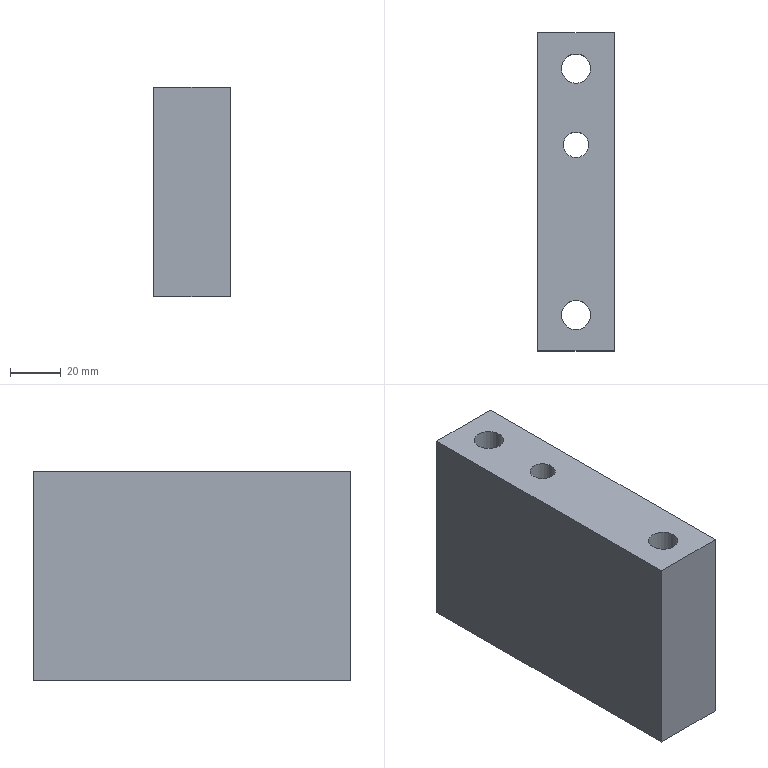Part | STEP file | lll_id3318_x_t | 1 solid | 32 faces | box 30 x 125 x 82.5 mm | volume 256192 mm3 | cylinder 20 | plane 12 | commonest cylinder face diameters 11.509 x2 18.007 x2 10 x1 13 x1 19.107 x1 19.147 x1
STEP:
#1=CARTESIAN_POINT('',(1968.,-173.338,0.));
#2=VERTEX_POINT('',#1);
#3=CARTESIAN_POINT('',(1963.552,-168.136,0.));
#4=VERTEX_POINT('',#3);
#5=CARTESIAN_POINT('',(1957.318,-177.969,0.));
#6=DIRECTION('',(0.,0.,1.));
#7=DIRECTION('',(-1.,0.,0.));
#8=AXIS2_PLACEMENT_3D('',#5,#6,#7);
#9=CIRCLE('',#8,11.642);
#10=EDGE_CURVE('',#2,#4,#9,.T.);
#11=ORIENTED_EDGE('',*,*,#10,.F.);
#12=CARTESIAN_POINT('',(1968.,-200.,0.));
#13=VERTEX_POINT('',#12);
#14=CARTESIAN_POINT('',(1968.,-4.,0.));
#15=DIRECTION('',(0.,-1.,0.));
#16=VECTOR('',#15,1.);
#17=LINE('',#14,#16);
#18=EDGE_CURVE('',#2,#13,#17,.T.);
#19=ORIENTED_EDGE('',*,*,#18,.T.);
#20=CARTESIAN_POINT('',(1938.,-200.,0.));
#21=VERTEX_POINT('',#20);
#22=CARTESIAN_POINT('',(1953.,-200.,0.));
#23=DIRECTION('',(-1.,0.,0.));
#24=VECTOR('',#23,1.);
#25=LINE('',#22,#24);
#26=EDGE_CURVE('',#13,#21,#25,.T.);
#27=ORIENTED_EDGE('',*,*,#26,.T.);
#28=CARTESIAN_POINT('',(1938.,-75.,0.));
#29=VERTEX_POINT('',#28);
#30=CARTESIAN_POINT('',(1938.,176.117,0.));
#31=DIRECTION('',(0.,-1.,0.));
#32=VECTOR('',#31,1.);
#33=LINE('',#30,#32);
#34=EDGE_CURVE('',#29,#21,#33,.T.);
#35=ORIENTED_EDGE('',*,*,#34,.F.);
#36=CARTESIAN_POINT('',(1968.,-75.,0.));
#37=VERTEX_POINT('',#36);
#38=CARTESIAN_POINT('',(1978.,-75.,0.));
#39=DIRECTION('',(1.,0.,0.));
#40=VECTOR('',#39,1.);
#41=LINE('',#38,#40);
#42=EDGE_CURVE('',#29,#37,#41,.T.);
#43=ORIENTED_EDGE('',*,*,#42,.T.);
#44=CARTESIAN_POINT('',(1968.,-127.474,0.));
#45=VERTEX_POINT('',#44);
#46=CARTESIAN_POINT('',(1968.,-4.,0.));
#47=DIRECTION('',(0.,-1.,0.));
#48=VECTOR('',#47,1.);
#49=LINE('',#46,#48);
#50=EDGE_CURVE('',#37,#45,#49,.T.);
#51=ORIENTED_EDGE('',*,*,#50,.T.);
#52=CARTESIAN_POINT('',(1965.589,-131.012,0.));
#53=VERTEX_POINT('',#52);
#54=CARTESIAN_POINT('',(1957.53,-122.929,0.));
#55=DIRECTION('',(0.,0.,-1.));
#56=DIRECTION('',(-1.,0.,0.));
#57=AXIS2_PLACEMENT_3D('',#54,#55,#56);
#58=CIRCLE('',#57,11.414);
#59=EDGE_CURVE('',#45,#53,#58,.T.);
#60=ORIENTED_EDGE('',*,*,#59,.T.);
#61=CARTESIAN_POINT('',(1964.899,-131.617,0.));
#62=VERTEX_POINT('',#61);
#63=CARTESIAN_POINT('',(1958.947,-124.145,0.));
#64=DIRECTION('',(0.,0.,-1.));
#65=DIRECTION('',(-1.,0.,0.));
#66=AXIS2_PLACEMENT_3D('',#63,#64,#65);
#67=CIRCLE('',#66,9.553);
#68=EDGE_CURVE('',#53,#62,#67,.T.);
#69=ORIENTED_EDGE('',*,*,#68,.T.);
#70=CARTESIAN_POINT('',(1964.24,-132.116,0.));
#71=VERTEX_POINT('',#70);
#72=CARTESIAN_POINT('',(1955.238,-119.534,0.));
#73=DIRECTION('',(0.,0.,-1.));
#74=DIRECTION('',(-1.,0.,0.));
#75=AXIS2_PLACEMENT_3D('',#72,#73,#74);
#76=CIRCLE('',#75,15.471);
#77=EDGE_CURVE('',#62,#71,#76,.T.);
#78=ORIENTED_EDGE('',*,*,#77,.T.);
#79=CARTESIAN_POINT('',(1963.503,-132.626,0.));
#80=VERTEX_POINT('',#79);
#81=CARTESIAN_POINT('',(1947.874,-109.242,0.));
#82=DIRECTION('',(0.,0.,-1.));
#83=DIRECTION('',(-1.,0.,0.));
#84=AXIS2_PLACEMENT_3D('',#81,#82,#83);
#85=CIRCLE('',#84,28.126);
#86=EDGE_CURVE('',#71,#80,#85,.T.);
#87=ORIENTED_EDGE('',*,*,#86,.T.);
#88=CARTESIAN_POINT('',(1962.795,-133.095,0.));
#89=VERTEX_POINT('',#88);
#90=CARTESIAN_POINT('',(1933.701,-88.407,0.));
#91=DIRECTION('',(0.,0.,-1.));
#92=DIRECTION('',(-1.,0.,0.));
#93=AXIS2_PLACEMENT_3D('',#90,#91,#92);
#94=CIRCLE('',#93,53.324);
#95=EDGE_CURVE('',#80,#89,#94,.T.);
#96=ORIENTED_EDGE('',*,*,#95,.T.);
#97=CARTESIAN_POINT('',(1949.008,-140.845,0.));
#98=VERTEX_POINT('',#97);
#99=CARTESIAN_POINT('',(2106.433,-52.349,0.));
#100=DIRECTION('',(-0.8717,-0.49,0.));
#101=VECTOR('',#100,1.);
#102=LINE('',#99,#101);
#103=EDGE_CURVE('',#89,#98,#102,.T.);
#104=ORIENTED_EDGE('',*,*,#103,.T.);
#105=CARTESIAN_POINT('',(1948.194,-141.368,0.));
#106=VERTEX_POINT('',#105);
#107=CARTESIAN_POINT('',(1961.447,-161.108,0.));
#108=DIRECTION('',(0.,0.,1.));
#109=DIRECTION('',(-1.,0.,0.));
#110=AXIS2_PLACEMENT_3D('',#107,#108,#109);
#111=CIRCLE('',#110,23.776);
#112=EDGE_CURVE('',#98,#106,#111,.T.);
#113=ORIENTED_EDGE('',*,*,#112,.T.);
#114=CARTESIAN_POINT('',(1947.304,-142.034,0.));
#115=VERTEX_POINT('',#114);
#116=CARTESIAN_POINT('',(1954.305,-150.47,0.));
#117=DIRECTION('',(0.,0.,1.));
#118=DIRECTION('',(-1.,0.,0.));
#119=AXIS2_PLACEMENT_3D('',#116,#117,#118);
#120=CIRCLE('',#119,10.964);
#121=EDGE_CURVE('',#106,#115,#120,.T.);
#122=ORIENTED_EDGE('',*,*,#121,.T.);
#123=CARTESIAN_POINT('',(1943.441,-151.267,0.));
#124=VERTEX_POINT('',#123);
#125=CARTESIAN_POINT('',(1954.482,-150.461,0.));
#126=DIRECTION('',(0.,0.,1.));
#127=DIRECTION('',(-1.,0.,0.));
#128=AXIS2_PLACEMENT_3D('',#125,#126,#127);
#129=CIRCLE('',#128,11.07);
#130=EDGE_CURVE('',#115,#124,#129,.T.);
#131=ORIENTED_EDGE('',*,*,#130,.T.);
#132=CARTESIAN_POINT('',(1945.982,-157.369,0.));
#133=VERTEX_POINT('',#132);
#134=CARTESIAN_POINT('',(1954.719,-150.151,0.));
#135=DIRECTION('',(0.,0.,-1.));
#136=DIRECTION('',(-1.,0.,0.));
#137=AXIS2_PLACEMENT_3D('',#134,#135,#136);
#138=CIRCLE('',#137,11.334);
#139=EDGE_CURVE('',#133,#124,#138,.T.);
#140=ORIENTED_EDGE('',*,*,#139,.F.);
#141=CARTESIAN_POINT('',(1947.347,-158.71,0.));
#142=VERTEX_POINT('',#141);
#143=CARTESIAN_POINT('',(1953.34,-151.245,0.));
#144=DIRECTION('',(0.,0.,-1.));
#145=DIRECTION('',(-1.,0.,0.));
#146=AXIS2_PLACEMENT_3D('',#143,#144,#145);
#147=CIRCLE('',#146,9.573);
#148=EDGE_CURVE('',#142,#133,#147,.T.);
#149=ORIENTED_EDGE('',*,*,#148,.F.);
#150=CARTESIAN_POINT('',(1948.15,-159.31,0.));
#151=VERTEX_POINT('',#150);
#152=CARTESIAN_POINT('',(1955.954,-148.02,0.));
#153=DIRECTION('',(0.,0.,-1.));
#154=DIRECTION('',(-1.,0.,0.));
#155=AXIS2_PLACEMENT_3D('',#152,#153,#154);
#156=CIRCLE('',#155,13.725);
#157=EDGE_CURVE('',#151,#142,#156,.T.);
#158=ORIENTED_EDGE('',*,*,#157,.F.);
#159=CARTESIAN_POINT('',(1948.955,-159.852,0.));
#160=VERTEX_POINT('',#159);
#161=CARTESIAN_POINT('',(1967.255,-131.809,0.));
#162=DIRECTION('',(0.,0.,-1.));
#163=DIRECTION('',(-1.,0.,0.));
#164=AXIS2_PLACEMENT_3D('',#161,#162,#163);
#165=CIRCLE('',#164,33.486);
#166=EDGE_CURVE('',#160,#151,#165,.T.);
#167=ORIENTED_EDGE('',*,*,#166,.F.);
#168=CARTESIAN_POINT('',(1962.805,-167.674,0.));
#169=VERTEX_POINT('',#168);
#170=CARTESIAN_POINT('',(1827.125,-91.053,0.));
#171=DIRECTION('',(-0.8708,0.4917,0.));
#172=VECTOR('',#171,1.);
#173=LINE('',#170,#172);
#174=EDGE_CURVE('',#169,#160,#173,.T.);
#175=ORIENTED_EDGE('',*,*,#174,.F.);
#176=CARTESIAN_POINT('',(1938.43,-207.856,0.));
#177=DIRECTION('',(0.,0.,1.));
#178=DIRECTION('',(-1.,0.,0.));
#179=AXIS2_PLACEMENT_3D('',#176,#177,#178);
#180=CIRCLE('',#179,46.998);
#181=EDGE_CURVE('',#4,#169,#180,.T.);
#182=ORIENTED_EDGE('',*,*,#181,.F.);
#183=EDGE_LOOP('',(#11,#19,#27,#35,#43,#51,#60,#69,#78,#87,#96,#104,#113,#122,#131,#140,#149,#158,#167,#175,#182));
#184=FACE_BOUND('',#183,.T.);
#185=CARTESIAN_POINT('',(1943.996,-89.,0.));
#186=VERTEX_POINT('',#185);
#187=CARTESIAN_POINT('',(1953.,-89.,0.));
#188=DIRECTION('',(0.,0.,-1.));
#189=DIRECTION('',(-1.,0.,0.));
#190=AXIS2_PLACEMENT_3D('',#187,#188,#189);
#191=CIRCLE('',#190,9.004);
#192=EDGE_CURVE('',#186,#186,#191,.T.);
#193=ORIENTED_EDGE('',*,*,#192,.F.);
#194=EDGE_LOOP('',(#193));
#195=FACE_BOUND('',#194,.T.);
#196=CARTESIAN_POINT('',(1943.996,-186.,0.));
#197=VERTEX_POINT('',#196);
#198=CARTESIAN_POINT('',(1953.,-186.,0.));
#199=DIRECTION('',(0.,0.,-1.));
#200=DIRECTION('',(-1.,0.,0.));
#201=AXIS2_PLACEMENT_3D('',#198,#199,#200);
#202=CIRCLE('',#201,9.004);
#203=EDGE_CURVE('',#197,#197,#202,.T.);
#204=ORIENTED_EDGE('',*,*,#203,.F.);
#205=EDGE_LOOP('',(#204));
#206=FACE_BOUND('',#205,.T.);
#207=CARTESIAN_POINT('',(1959.5,-119.,0.));
#208=VERTEX_POINT('',#207);
#209=CARTESIAN_POINT('',(1953.,-119.,0.));
#210=DIRECTION('',(0.,0.,1.));
#211=DIRECTION('',(1.,0.,0.));
#212=AXIS2_PLACEMENT_3D('',#209,#210,#211);
#213=CIRCLE('',#212,6.5);
#214=EDGE_CURVE('',#208,#208,#213,.T.);
#215=ORIENTED_EDGE('',*,*,#214,.T.);
#216=EDGE_LOOP('',(#215));
#217=FACE_BOUND('',#216,.T.);
#218=CARTESIAN_POINT('',(1978.,176.117,0.));
#219=DIRECTION('',(0.,0.,-1.));
#220=DIRECTION('',(-1.,0.,0.));
#221=AXIS2_PLACEMENT_3D('',#218,#219,#220);
#222=PLANE('',#221);
#223=ADVANCED_FACE('',(#184,#195,#206,#217),#222,.T.);
#224=CARTESIAN_POINT('',(1962.004,-186.,52.5));
#225=VERTEX_POINT('',#224);
#226=CARTESIAN_POINT('',(1953.,-186.,52.5));
#227=DIRECTION('',(0.,0.,1.));
#228=DIRECTION('',(1.,0.,0.));
#229=AXIS2_PLACEMENT_3D('',#226,#227,#228);
#230=CIRCLE('',#229,9.004);
#231=EDGE_CURVE('',#225,#225,#230,.T.);
#232=ORIENTED_EDGE('',*,*,#231,.T.);
#233=EDGE_LOOP('',(#232));
#234=FACE_BOUND('',#233,.T.);
#235=ORIENTED_EDGE('',*,*,#203,.T.);
#236=EDGE_LOOP('',(#235));
#237=FACE_BOUND('',#236,.T.);
#238=CARTESIAN_POINT('',(1953.,-186.,2.5));
#239=DIRECTION('',(0.,0.,1.));
#240=DIRECTION('',(1.,0.,0.));
#241=AXIS2_PLACEMENT_3D('',#238,#239,#240);
#242=CYLINDRICAL_SURFACE('',#241,9.004);
#243=ADVANCED_FACE('',(#234,#237),#242,.F.);
#244=CARTESIAN_POINT('',(1962.004,-89.,52.5));
#245=VERTEX_POINT('',#244);
#246=CARTESIAN_POINT('',(1953.,-89.,52.5));
#247=DIRECTION('',(0.,0.,1.));
#248=DIRECTION('',(1.,0.,0.));
#249=AXIS2_PLACEMENT_3D('',#246,#247,#248);
#250=CIRCLE('',#249,9.004);
#251=EDGE_CURVE('',#245,#245,#250,.T.);
#252=ORIENTED_EDGE('',*,*,#251,.T.);
#253=EDGE_LOOP('',(#252));
#254=FACE_BOUND('',#253,.T.);
#255=ORIENTED_EDGE('',*,*,#192,.T.);
#256=EDGE_LOOP('',(#255));
#257=FACE_BOUND('',#256,.T.);
#258=CARTESIAN_POINT('',(1953.,-89.,2.5));
#259=DIRECTION('',(0.,0.,1.));
#260=DIRECTION('',(1.,0.,0.));
#261=AXIS2_PLACEMENT_3D('',#258,#259,#260);
#262=CYLINDRICAL_SURFACE('',#261,9.004);
#263=ADVANCED_FACE('',(#254,#257),#262,.F.);
#264=CARTESIAN_POINT('',(1968.,-127.474,17.));
#265=VERTEX_POINT('',#264);
#266=CARTESIAN_POINT('',(1968.,-127.474,2.5));
#267=DIRECTION('',(0.,0.,1.));
#268=VECTOR('',#267,1.);
#269=LINE('',#266,#268);
#270=EDGE_CURVE('',#45,#265,#269,.T.);
#271=ORIENTED_EDGE('',*,*,#270,.F.);
#272=ORIENTED_EDGE('',*,*,#50,.F.);
#273=CARTESIAN_POINT('',(1968.,-75.,82.5));
#274=VERTEX_POINT('',#273);
#275=CARTESIAN_POINT('',(1968.,-75.,40.));
#276=DIRECTION('',(0.,0.,-1.));
#277=VECTOR('',#276,1.);
#278=LINE('',#275,#277);
#279=EDGE_CURVE('',#274,#37,#278,.T.);
#280=ORIENTED_EDGE('',*,*,#279,.F.);
#281=CARTESIAN_POINT('',(1968.,-200.,82.5));
#282=VERTEX_POINT('',#281);
#283=CARTESIAN_POINT('',(1968.,-4.,82.5));
#284=DIRECTION('',(0.,1.,0.));
#285=VECTOR('',#284,1.);
#286=LINE('',#283,#285);
#287=EDGE_CURVE('',#282,#274,#286,.T.);
#288=ORIENTED_EDGE('',*,*,#287,.F.);
#289=CARTESIAN_POINT('',(1968.,-200.,-652.5));
#290=DIRECTION('',(0.,0.,-1.));
#291=VECTOR('',#290,1.);
#292=LINE('',#289,#291);
#293=EDGE_CURVE('',#282,#13,#292,.T.);
#294=ORIENTED_EDGE('',*,*,#293,.T.);
#295=ORIENTED_EDGE('',*,*,#18,.F.);
#296=CARTESIAN_POINT('',(1968.,-173.338,17.));
#297=VERTEX_POINT('',#296);
#298=CARTESIAN_POINT('',(1968.,-173.338,5.5));
#299=DIRECTION('',(0.,0.,-1.));
#300=VECTOR('',#299,1.);
#301=LINE('',#298,#300);
#302=EDGE_CURVE('',#297,#2,#301,.T.);
#303=ORIENTED_EDGE('',*,*,#302,.F.);
#304=CARTESIAN_POINT('',(1968.,-4.,17.));
#305=DIRECTION('',(0.,-1.,0.));
#306=VECTOR('',#305,1.);
#307=LINE('',#304,#306);
#308=EDGE_CURVE('',#265,#297,#307,.T.);
#309=ORIENTED_EDGE('',*,*,#308,.F.);
#310=EDGE_LOOP('',(#271,#272,#280,#288,#294,#295,#303,#309));
#311=FACE_OUTER_BOUND('',#310,.T.);
#312=CARTESIAN_POINT('',(1968.,-4.,-652.5));
#313=DIRECTION('',(-1.,0.,0.));
#314=DIRECTION('',(0.,0.,1.));
#315=AXIS2_PLACEMENT_3D('',#312,#313,#314);
#316=PLANE('',#315);
#317=ADVANCED_FACE('',(#311),#316,.F.);
#318=CARTESIAN_POINT('',(1958.755,-186.,82.5));
#319=VERTEX_POINT('',#318);
#320=CARTESIAN_POINT('',(1953.,-186.,82.5));
#321=DIRECTION('',(0.,0.,1.));
#322=DIRECTION('',(1.,0.,0.));
#323=AXIS2_PLACEMENT_3D('',#320,#321,#322);
#324=CIRCLE('',#323,5.755);
#325=EDGE_CURVE('',#319,#319,#324,.T.);
#326=ORIENTED_EDGE('',*,*,#325,.F.);
#327=EDGE_LOOP('',(#326));
#328=FACE_BOUND('',#327,.T.);
#329=CARTESIAN_POINT('',(1958.755,-89.,82.5));
#330=VERTEX_POINT('',#329);
#331=CARTESIAN_POINT('',(1953.,-89.,82.5));
#332=DIRECTION('',(0.,0.,1.));
#333=DIRECTION('',(1.,0.,0.));
#334=AXIS2_PLACEMENT_3D('',#331,#332,#333);
#335=CIRCLE('',#334,5.755);
#336=EDGE_CURVE('',#330,#330,#335,.T.);
#337=ORIENTED_EDGE('',*,*,#336,.F.);
#338=EDGE_LOOP('',(#337));
#339=FACE_BOUND('',#338,.T.);
#340=CARTESIAN_POINT('',(1958.,-119.,82.5));
#341=VERTEX_POINT('',#340);
#342=CARTESIAN_POINT('',(1953.,-119.,82.5));
#343=DIRECTION('',(0.,0.,1.));
#344=DIRECTION('',(1.,0.,0.));
#345=AXIS2_PLACEMENT_3D('',#342,#343,#344);
#346=CIRCLE('',#345,5.);
#347=EDGE_CURVE('',#341,#341,#346,.T.);
#348=ORIENTED_EDGE('',*,*,#347,.F.);
#349=EDGE_LOOP('',(#348));
#350=FACE_BOUND('',#349,.T.);
#351=CARTESIAN_POINT('',(1938.,-200.,82.5));
#352=VERTEX_POINT('',#351);
#353=CARTESIAN_POINT('',(1978.,-200.,82.5));
#354=DIRECTION('',(-1.,0.,0.));
#355=VECTOR('',#354,1.);
#356=LINE('',#353,#355);
#357=EDGE_CURVE('',#282,#352,#356,.T.);
#358=ORIENTED_EDGE('',*,*,#357,.F.);
#359=ORIENTED_EDGE('',*,*,#287,.T.);
#360=CARTESIAN_POINT('',(1938.,-75.,82.5));
#361=VERTEX_POINT('',#360);
#362=CARTESIAN_POINT('',(1978.,-75.,82.5));
#363=DIRECTION('',(1.,0.,0.));
#364=VECTOR('',#363,1.);
#365=LINE('',#362,#364);
#366=EDGE_CURVE('',#361,#274,#365,.T.);
#367=ORIENTED_EDGE('',*,*,#366,.F.);
#368=CARTESIAN_POINT('',(1938.,-4.,82.5));
#369=DIRECTION('',(0.,1.,0.));
#370=VECTOR('',#369,1.);
#371=LINE('',#368,#370);
#372=EDGE_CURVE('',#352,#361,#371,.T.);
#373=ORIENTED_EDGE('',*,*,#372,.F.);
#374=EDGE_LOOP('',(#358,#359,#367,#373));
#375=FACE_BOUND('',#374,.T.);
#376=CARTESIAN_POINT('',(1978.,-236.117,82.5));
#377=DIRECTION('',(0.,0.,1.));
#378=DIRECTION('',(1.,0.,0.));
#379=AXIS2_PLACEMENT_3D('',#376,#377,#378);
#380=PLANE('',#379);
#381=ADVANCED_FACE('',(#328,#339,#350,#375),#380,.T.);
#382=CARTESIAN_POINT('',(1938.,-200.,40.));
#383=DIRECTION('',(0.,0.,1.));
#384=VECTOR('',#383,1.);
#385=LINE('',#382,#384);
#386=EDGE_CURVE('',#21,#352,#385,.T.);
#387=ORIENTED_EDGE('',*,*,#386,.T.);
#388=ORIENTED_EDGE('',*,*,#372,.T.);
#389=CARTESIAN_POINT('',(1938.,-75.,-652.5));
#390=DIRECTION('',(0.,0.,1.));
#391=VECTOR('',#390,1.);
#392=LINE('',#389,#391);
#393=EDGE_CURVE('',#29,#361,#392,.T.);
#394=ORIENTED_EDGE('',*,*,#393,.F.);
#395=ORIENTED_EDGE('',*,*,#34,.T.);
#396=EDGE_LOOP('',(#387,#388,#394,#395));
#397=FACE_OUTER_BOUND('',#396,.T.);
#398=CARTESIAN_POINT('',(1938.,-4.,-652.5));
#399=DIRECTION('',(-1.,0.,0.));
#400=DIRECTION('',(0.,0.,1.));
#401=AXIS2_PLACEMENT_3D('',#398,#399,#400);
#402=PLANE('',#401);
#403=ADVANCED_FACE('',(#397),#402,.T.);
#404=ORIENTED_EDGE('',*,*,#42,.F.);
#405=ORIENTED_EDGE('',*,*,#393,.T.);
#406=ORIENTED_EDGE('',*,*,#366,.T.);
#407=ORIENTED_EDGE('',*,*,#279,.T.);
#408=EDGE_LOOP('',(#404,#405,#406,#407));
#409=FACE_OUTER_BOUND('',#408,.T.);
#410=CARTESIAN_POINT('',(2239.,-75.,40.));
#411=DIRECTION('',(0.,-1.,0.));
#412=DIRECTION('',(0.,0.,-1.));
#413=AXIS2_PLACEMENT_3D('',#410,#411,#412);
#414=PLANE('',#413);
#415=ADVANCED_FACE('',(#409),#414,.F.);
#416=ORIENTED_EDGE('',*,*,#357,.T.);
#417=ORIENTED_EDGE('',*,*,#386,.F.);
#418=ORIENTED_EDGE('',*,*,#26,.F.);
#419=ORIENTED_EDGE('',*,*,#293,.F.);
#420=EDGE_LOOP('',(#416,#417,#418,#419));
#421=FACE_OUTER_BOUND('',#420,.T.);
#422=CARTESIAN_POINT('',(1953.,-200.,40.));
#423=DIRECTION('',(0.,1.,0.));
#424=DIRECTION('',(0.,0.,1.));
#425=AXIS2_PLACEMENT_3D('',#422,#423,#424);
#426=PLANE('',#425);
#427=ADVANCED_FACE('',(#421),#426,.F.);
#428=ORIENTED_EDGE('',*,*,#270,.T.);
#429=CARTESIAN_POINT('',(1965.589,-131.012,17.));
#430=VERTEX_POINT('',#429);
#431=CARTESIAN_POINT('',(1957.53,-122.929,17.));
#432=DIRECTION('',(0.,0.,1.));
#433=DIRECTION('',(-1.,0.,0.));
#434=AXIS2_PLACEMENT_3D('',#431,#432,#433);
#435=CIRCLE('',#434,11.414);
#436=EDGE_CURVE('',#430,#265,#435,.T.);
#437=ORIENTED_EDGE('',*,*,#436,.F.);
#438=CARTESIAN_POINT('',(1965.589,-131.012,5.5));
#439=DIRECTION('',(0.,0.,-1.));
#440=VECTOR('',#439,1.);
#441=LINE('',#438,#440);
#442=EDGE_CURVE('',#430,#53,#441,.T.);
#443=ORIENTED_EDGE('',*,*,#442,.T.);
#444=ORIENTED_EDGE('',*,*,#59,.F.);
#445=EDGE_LOOP('',(#428,#437,#443,#444));
#446=FACE_OUTER_BOUND('',#445,.T.);
#447=CARTESIAN_POINT('',(1957.53,-122.929,2.5));
#448=DIRECTION('',(0.,0.,-1.));
#449=DIRECTION('',(-1.,0.,0.));
#450=AXIS2_PLACEMENT_3D('',#447,#448,#449);
#451=CYLINDRICAL_SURFACE('',#450,11.414);
#452=ADVANCED_FACE('',(#446),#451,.T.);
#453=ORIENTED_EDGE('',*,*,#302,.T.);
#454=ORIENTED_EDGE('',*,*,#10,.T.);
#455=CARTESIAN_POINT('',(1963.552,-168.136,17.));
#456=VERTEX_POINT('',#455);
#457=CARTESIAN_POINT('',(1963.552,-168.136,2.5));
#458=DIRECTION('',(0.,0.,-1.));
#459=VECTOR('',#458,1.);
#460=LINE('',#457,#459);
#461=EDGE_CURVE('',#456,#4,#460,.T.);
#462=ORIENTED_EDGE('',*,*,#461,.F.);
#463=CARTESIAN_POINT('',(1957.318,-177.969,17.));
#464=DIRECTION('',(0.,0.,-1.));
#465=DIRECTION('',(-1.,0.,0.));
#466=AXIS2_PLACEMENT_3D('',#463,#464,#465);
#467=CIRCLE('',#466,11.642);
#468=EDGE_CURVE('',#456,#297,#467,.T.);
#469=ORIENTED_EDGE('',*,*,#468,.T.);
#470=EDGE_LOOP('',(#453,#454,#462,#469));
#471=FACE_OUTER_BOUND('',#470,.T.);
#472=CARTESIAN_POINT('',(1957.318,-177.969,2.5));
#473=DIRECTION('',(0.,0.,-1.));
#474=DIRECTION('',(-1.,0.,0.));
#475=AXIS2_PLACEMENT_3D('',#472,#473,#474);
#476=CYLINDRICAL_SURFACE('',#475,11.642);
#477=ADVANCED_FACE('',(#471),#476,.T.);
#478=ORIENTED_EDGE('',*,*,#308,.T.);
#479=ORIENTED_EDGE('',*,*,#468,.F.);
#480=CARTESIAN_POINT('',(1962.805,-167.674,17.));
#481=VERTEX_POINT('',#480);
#482=CARTESIAN_POINT('',(1938.43,-207.856,17.));
#483=DIRECTION('',(0.,0.,-1.));
#484=DIRECTION('',(-1.,0.,0.));
#485=AXIS2_PLACEMENT_3D('',#482,#483,#484);
#486=CIRCLE('',#485,46.998);
#487=EDGE_CURVE('',#481,#456,#486,.T.);
#488=ORIENTED_EDGE('',*,*,#487,.F.);
#489=CARTESIAN_POINT('',(1948.955,-159.852,17.));
#490=VERTEX_POINT('',#489);
#491=CARTESIAN_POINT('',(1962.845,-167.696,17.));
#492=DIRECTION('',(0.8708,-0.4917,0.));
#493=VECTOR('',#492,1.);
#494=LINE('',#491,#493);
#495=EDGE_CURVE('',#490,#481,#494,.T.);
#496=ORIENTED_EDGE('',*,*,#495,.F.);
#497=CARTESIAN_POINT('',(1948.15,-159.31,17.));
#498=VERTEX_POINT('',#497);
#499=CARTESIAN_POINT('',(1967.255,-131.809,17.));
#500=DIRECTION('',(0.,0.,1.));
#501=DIRECTION('',(-1.,0.,0.));
#502=AXIS2_PLACEMENT_3D('',#499,#500,#501);
#503=CIRCLE('',#502,33.486);
#504=EDGE_CURVE('',#498,#490,#503,.T.);
#505=ORIENTED_EDGE('',*,*,#504,.F.);
#506=CARTESIAN_POINT('',(1947.347,-158.71,17.));
#507=VERTEX_POINT('',#506);
#508=CARTESIAN_POINT('',(1955.954,-148.02,17.));
#509=DIRECTION('',(0.,0.,1.));
#510=DIRECTION('',(-1.,0.,0.));
#511=AXIS2_PLACEMENT_3D('',#508,#509,#510);
#512=CIRCLE('',#511,13.725);
#513=EDGE_CURVE('',#507,#498,#512,.T.);
#514=ORIENTED_EDGE('',*,*,#513,.F.);
#515=CARTESIAN_POINT('',(1945.982,-157.369,17.));
#516=VERTEX_POINT('',#515);
#517=CARTESIAN_POINT('',(1953.34,-151.245,17.));
#518=DIRECTION('',(0.,0.,1.));
#519=DIRECTION('',(-1.,0.,0.));
#520=AXIS2_PLACEMENT_3D('',#517,#518,#519);
#521=CIRCLE('',#520,9.573);
#522=EDGE_CURVE('',#516,#507,#521,.T.);
#523=ORIENTED_EDGE('',*,*,#522,.F.);
#524=CARTESIAN_POINT('',(1943.441,-151.267,17.));
#525=VERTEX_POINT('',#524);
#526=CARTESIAN_POINT('',(1954.719,-150.151,17.));
#527=DIRECTION('',(0.,0.,1.));
#528=DIRECTION('',(-1.,0.,0.));
#529=AXIS2_PLACEMENT_3D('',#526,#527,#528);
#530=CIRCLE('',#529,11.334);
#531=EDGE_CURVE('',#525,#516,#530,.T.);
#532=ORIENTED_EDGE('',*,*,#531,.F.);
#533=CARTESIAN_POINT('',(1947.304,-142.034,17.));
#534=VERTEX_POINT('',#533);
#535=CARTESIAN_POINT('',(1954.482,-150.461,17.));
#536=DIRECTION('',(0.,0.,-1.));
#537=DIRECTION('',(-1.,0.,0.));
#538=AXIS2_PLACEMENT_3D('',#535,#536,#537);
#539=CIRCLE('',#538,11.07);
#540=EDGE_CURVE('',#525,#534,#539,.T.);
#541=ORIENTED_EDGE('',*,*,#540,.T.);
#542=CARTESIAN_POINT('',(1948.194,-141.368,17.));
#543=VERTEX_POINT('',#542);
#544=CARTESIAN_POINT('',(1954.305,-150.47,17.));
#545=DIRECTION('',(0.,0.,-1.));
#546=DIRECTION('',(-1.,0.,0.));
#547=AXIS2_PLACEMENT_3D('',#544,#545,#546);
#548=CIRCLE('',#547,10.964);
#549=EDGE_CURVE('',#534,#543,#548,.T.);
#550=ORIENTED_EDGE('',*,*,#549,.T.);
#551=CARTESIAN_POINT('',(1949.008,-140.845,17.));
#552=VERTEX_POINT('',#551);
#553=CARTESIAN_POINT('',(1961.447,-161.108,17.));
#554=DIRECTION('',(0.,0.,-1.));
#555=DIRECTION('',(-1.,0.,0.));
#556=AXIS2_PLACEMENT_3D('',#553,#554,#555);
#557=CIRCLE('',#556,23.776);
#558=EDGE_CURVE('',#543,#552,#557,.T.);
#559=ORIENTED_EDGE('',*,*,#558,.T.);
#560=CARTESIAN_POINT('',(1962.795,-133.095,17.));
#561=VERTEX_POINT('',#560);
#562=CARTESIAN_POINT('',(1962.879,-133.048,17.));
#563=DIRECTION('',(0.8717,0.49,0.));
#564=VECTOR('',#563,1.);
#565=LINE('',#562,#564);
#566=EDGE_CURVE('',#552,#561,#565,.T.);
#567=ORIENTED_EDGE('',*,*,#566,.T.);
#568=CARTESIAN_POINT('',(1963.503,-132.626,17.));
#569=VERTEX_POINT('',#568);
#570=CARTESIAN_POINT('',(1933.701,-88.407,17.));
#571=DIRECTION('',(0.,0.,1.));
#572=DIRECTION('',(-1.,0.,0.));
#573=AXIS2_PLACEMENT_3D('',#570,#571,#572);
#574=CIRCLE('',#573,53.324);
#575=EDGE_CURVE('',#561,#569,#574,.T.);
#576=ORIENTED_EDGE('',*,*,#575,.T.);
#577=CARTESIAN_POINT('',(1964.24,-132.116,17.));
#578=VERTEX_POINT('',#577);
#579=CARTESIAN_POINT('',(1947.874,-109.242,17.));
#580=DIRECTION('',(0.,0.,1.));
#581=DIRECTION('',(-1.,0.,0.));
#582=AXIS2_PLACEMENT_3D('',#579,#580,#581);
#583=CIRCLE('',#582,28.126);
#584=EDGE_CURVE('',#569,#578,#583,.T.);
#585=ORIENTED_EDGE('',*,*,#584,.T.);
#586=CARTESIAN_POINT('',(1964.899,-131.617,17.));
#587=VERTEX_POINT('',#586);
#588=CARTESIAN_POINT('',(1955.238,-119.534,17.));
#589=DIRECTION('',(0.,0.,1.));
#590=DIRECTION('',(-1.,0.,0.));
#591=AXIS2_PLACEMENT_3D('',#588,#589,#590);
#592=CIRCLE('',#591,15.471);
#593=EDGE_CURVE('',#578,#587,#592,.T.);
#594=ORIENTED_EDGE('',*,*,#593,.T.);
#595=CARTESIAN_POINT('',(1958.947,-124.145,17.));
#596=DIRECTION('',(0.,0.,1.));
#597=DIRECTION('',(-1.,0.,0.));
#598=AXIS2_PLACEMENT_3D('',#595,#596,#597);
#599=CIRCLE('',#598,9.553);
#600=EDGE_CURVE('',#587,#430,#599,.T.);
#601=ORIENTED_EDGE('',*,*,#600,.T.);
#602=ORIENTED_EDGE('',*,*,#436,.T.);
#603=EDGE_LOOP('',(#478,#479,#488,#496,#505,#514,#523,#532,#541,#550,#559,#567,#576,#585,#594,#601,#602));
#604=FACE_OUTER_BOUND('',#603,.T.);
#605=CARTESIAN_POINT('',(12867.883,-13712.786,17.));
#606=DIRECTION('',(0.,0.,-1.));
#607=DIRECTION('',(-1.,0.,0.));
#608=AXIS2_PLACEMENT_3D('',#605,#606,#607);
#609=PLANE('',#608);
#610=ADVANCED_FACE('',(#604),#609,.T.);
#611=ORIENTED_EDGE('',*,*,#68,.F.);
#612=ORIENTED_EDGE('',*,*,#442,.F.);
#613=ORIENTED_EDGE('',*,*,#600,.F.);
#614=CARTESIAN_POINT('',(1964.899,-131.617,5.5));
#615=DIRECTION('',(0.,0.,-1.));
#616=VECTOR('',#615,1.);
#617=LINE('',#614,#616);
#618=EDGE_CURVE('',#587,#62,#617,.T.);
#619=ORIENTED_EDGE('',*,*,#618,.T.);
#620=EDGE_LOOP('',(#611,#612,#613,#619));
#621=FACE_OUTER_BOUND('',#620,.T.);
#622=CARTESIAN_POINT('',(1958.947,-124.145,2.5));
#623=DIRECTION('',(0.,0.,-1.));
#624=DIRECTION('',(-1.,0.,0.));
#625=AXIS2_PLACEMENT_3D('',#622,#623,#624);
#626=CYLINDRICAL_SURFACE('',#625,9.553);
#627=ADVANCED_FACE('',(#621),#626,.T.);
#628=ORIENTED_EDGE('',*,*,#77,.F.);
#629=ORIENTED_EDGE('',*,*,#618,.F.);
#630=ORIENTED_EDGE('',*,*,#593,.F.);
#631=CARTESIAN_POINT('',(1964.24,-132.116,2.5));
#632=DIRECTION('',(0.,0.,-1.));
#633=VECTOR('',#632,1.);
#634=LINE('',#631,#633);
#635=EDGE_CURVE('',#578,#71,#634,.T.);
#636=ORIENTED_EDGE('',*,*,#635,.T.);
#637=EDGE_LOOP('',(#628,#629,#630,#636));
#638=FACE_OUTER_BOUND('',#637,.T.);
#639=CARTESIAN_POINT('',(1955.238,-119.534,2.5));
#640=DIRECTION('',(0.,0.,-1.));
#641=DIRECTION('',(-1.,0.,0.));
#642=AXIS2_PLACEMENT_3D('',#639,#640,#641);
#643=CYLINDRICAL_SURFACE('',#642,15.471);
#644=ADVANCED_FACE('',(#638),#643,.T.);
#645=ORIENTED_EDGE('',*,*,#86,.F.);
#646=ORIENTED_EDGE('',*,*,#635,.F.);
#647=ORIENTED_EDGE('',*,*,#584,.F.);
#648=CARTESIAN_POINT('',(1963.503,-132.626,5.5));
#649=DIRECTION('',(0.,0.,-1.));
#650=VECTOR('',#649,1.);
#651=LINE('',#648,#650);
#652=EDGE_CURVE('',#569,#80,#651,.T.);
#653=ORIENTED_EDGE('',*,*,#652,.T.);
#654=EDGE_LOOP('',(#645,#646,#647,#653));
#655=FACE_OUTER_BOUND('',#654,.T.);
#656=CARTESIAN_POINT('',(1947.874,-109.242,2.5));
#657=DIRECTION('',(0.,0.,-1.));
#658=DIRECTION('',(-1.,0.,0.));
#659=AXIS2_PLACEMENT_3D('',#656,#657,#658);
#660=CYLINDRICAL_SURFACE('',#659,28.126);
#661=ADVANCED_FACE('',(#655),#660,.T.);
#662=ORIENTED_EDGE('',*,*,#95,.F.);
#663=ORIENTED_EDGE('',*,*,#652,.F.);
#664=ORIENTED_EDGE('',*,*,#575,.F.);
#665=CARTESIAN_POINT('',(1962.795,-133.095,5.5));
#666=DIRECTION('',(0.,0.,-1.));
#667=VECTOR('',#666,1.);
#668=LINE('',#665,#667);
#669=EDGE_CURVE('',#561,#89,#668,.T.);
#670=ORIENTED_EDGE('',*,*,#669,.T.);
#671=EDGE_LOOP('',(#662,#663,#664,#670));
#672=FACE_OUTER_BOUND('',#671,.T.);
#673=CARTESIAN_POINT('',(1933.701,-88.407,2.5));
#674=DIRECTION('',(0.,0.,-1.));
#675=DIRECTION('',(-1.,0.,0.));
#676=AXIS2_PLACEMENT_3D('',#673,#674,#675);
#677=CYLINDRICAL_SURFACE('',#676,53.324);
#678=ADVANCED_FACE('',(#672),#677,.T.);
#679=ORIENTED_EDGE('',*,*,#103,.F.);
#680=ORIENTED_EDGE('',*,*,#669,.F.);
#681=ORIENTED_EDGE('',*,*,#566,.F.);
#682=CARTESIAN_POINT('',(1949.008,-140.845,5.5));
#683=DIRECTION('',(0.,0.,-1.));
#684=VECTOR('',#683,1.);
#685=LINE('',#682,#684);
#686=EDGE_CURVE('',#552,#98,#685,.T.);
#687=ORIENTED_EDGE('',*,*,#686,.T.);
#688=EDGE_LOOP('',(#679,#680,#681,#687));
#689=FACE_OUTER_BOUND('',#688,.T.);
#690=CARTESIAN_POINT('',(1962.879,-133.048,2.5));
#691=DIRECTION('',(0.49,-0.8717,0.));
#692=DIRECTION('',(-0.8717,-0.49,0.));
#693=AXIS2_PLACEMENT_3D('',#690,#691,#692);
#694=PLANE('',#693);
#695=ADVANCED_FACE('',(#689),#694,.T.);
#696=ORIENTED_EDGE('',*,*,#112,.F.);
#697=ORIENTED_EDGE('',*,*,#686,.F.);
#698=ORIENTED_EDGE('',*,*,#558,.F.);
#699=CARTESIAN_POINT('',(1948.194,-141.368,2.5));
#700=DIRECTION('',(0.,0.,-1.));
#701=VECTOR('',#700,1.);
#702=LINE('',#699,#701);
#703=EDGE_CURVE('',#543,#106,#702,.T.);
#704=ORIENTED_EDGE('',*,*,#703,.T.);
#705=EDGE_LOOP('',(#696,#697,#698,#704));
#706=FACE_OUTER_BOUND('',#705,.T.);
#707=CARTESIAN_POINT('',(1961.447,-161.108,2.5));
#708=DIRECTION('',(0.,0.,-1.));
#709=DIRECTION('',(-1.,0.,0.));
#710=AXIS2_PLACEMENT_3D('',#707,#708,#709);
#711=CYLINDRICAL_SURFACE('',#710,23.776);
#712=ADVANCED_FACE('',(#706),#711,.F.);
#713=ORIENTED_EDGE('',*,*,#121,.F.);
#714=ORIENTED_EDGE('',*,*,#703,.F.);
#715=ORIENTED_EDGE('',*,*,#549,.F.);
#716=CARTESIAN_POINT('',(1947.304,-142.034,5.5));
#717=DIRECTION('',(0.,0.,-1.));
#718=VECTOR('',#717,1.);
#719=LINE('',#716,#718);
#720=EDGE_CURVE('',#534,#115,#719,.T.);
#721=ORIENTED_EDGE('',*,*,#720,.T.);
#722=EDGE_LOOP('',(#713,#714,#715,#721));
#723=FACE_OUTER_BOUND('',#722,.T.);
#724=CARTESIAN_POINT('',(1954.305,-150.47,2.5));
#725=DIRECTION('',(0.,0.,-1.));
#726=DIRECTION('',(-1.,0.,0.));
#727=AXIS2_PLACEMENT_3D('',#724,#725,#726);
#728=CYLINDRICAL_SURFACE('',#727,10.964);
#729=ADVANCED_FACE('',(#723),#728,.F.);
#730=ORIENTED_EDGE('',*,*,#130,.F.);
#731=ORIENTED_EDGE('',*,*,#720,.F.);
#732=ORIENTED_EDGE('',*,*,#540,.F.);
#733=CARTESIAN_POINT('',(1943.441,-151.267,5.5));
#734=DIRECTION('',(0.,0.,-1.));
#735=VECTOR('',#734,1.);
#736=LINE('',#733,#735);
#737=EDGE_CURVE('',#525,#124,#736,.T.);
#738=ORIENTED_EDGE('',*,*,#737,.T.);
#739=EDGE_LOOP('',(#730,#731,#732,#738));
#740=FACE_OUTER_BOUND('',#739,.T.);
#741=CARTESIAN_POINT('',(1954.482,-150.461,2.5));
#742=DIRECTION('',(0.,0.,-1.));
#743=DIRECTION('',(-1.,0.,0.));
#744=AXIS2_PLACEMENT_3D('',#741,#742,#743);
#745=CYLINDRICAL_SURFACE('',#744,11.07);
#746=ADVANCED_FACE('',(#740),#745,.F.);
#747=ORIENTED_EDGE('',*,*,#139,.T.);
#748=ORIENTED_EDGE('',*,*,#737,.F.);
#749=ORIENTED_EDGE('',*,*,#531,.T.);
#750=CARTESIAN_POINT('',(1945.982,-157.369,5.5));
#751=DIRECTION('',(0.,0.,-1.));
#752=VECTOR('',#751,1.);
#753=LINE('',#750,#752);
#754=EDGE_CURVE('',#516,#133,#753,.T.);
#755=ORIENTED_EDGE('',*,*,#754,.T.);
#756=EDGE_LOOP('',(#747,#748,#749,#755));
#757=FACE_OUTER_BOUND('',#756,.T.);
#758=CARTESIAN_POINT('',(1954.719,-150.151,2.5));
#759=DIRECTION('',(0.,0.,-1.));
#760=DIRECTION('',(-1.,0.,0.));
#761=AXIS2_PLACEMENT_3D('',#758,#759,#760);
#762=CYLINDRICAL_SURFACE('',#761,11.334);
#763=ADVANCED_FACE('',(#757),#762,.F.);
#764=ORIENTED_EDGE('',*,*,#148,.T.);
#765=ORIENTED_EDGE('',*,*,#754,.F.);
#766=ORIENTED_EDGE('',*,*,#522,.T.);
#767=CARTESIAN_POINT('',(1947.347,-158.71,5.5));
#768=DIRECTION('',(0.,0.,-1.));
#769=VECTOR('',#768,1.);
#770=LINE('',#767,#769);
#771=EDGE_CURVE('',#507,#142,#770,.T.);
#772=ORIENTED_EDGE('',*,*,#771,.T.);
#773=EDGE_LOOP('',(#764,#765,#766,#772));
#774=FACE_OUTER_BOUND('',#773,.T.);
#775=CARTESIAN_POINT('',(1953.34,-151.245,2.5));
#776=DIRECTION('',(0.,0.,-1.));
#777=DIRECTION('',(-1.,0.,0.));
#778=AXIS2_PLACEMENT_3D('',#775,#776,#777);
#779=CYLINDRICAL_SURFACE('',#778,9.573);
#780=ADVANCED_FACE('',(#774),#779,.F.);
#781=ORIENTED_EDGE('',*,*,#157,.T.);
#782=ORIENTED_EDGE('',*,*,#771,.F.);
#783=ORIENTED_EDGE('',*,*,#513,.T.);
#784=CARTESIAN_POINT('',(1948.15,-159.31,5.5));
#785=DIRECTION('',(0.,0.,-1.));
#786=VECTOR('',#785,1.);
#787=LINE('',#784,#786);
#788=EDGE_CURVE('',#498,#151,#787,.T.);
#789=ORIENTED_EDGE('',*,*,#788,.T.);
#790=EDGE_LOOP('',(#781,#782,#783,#789));
#791=FACE_OUTER_BOUND('',#790,.T.);
#792=CARTESIAN_POINT('',(1955.954,-148.02,2.5));
#793=DIRECTION('',(0.,0.,-1.));
#794=DIRECTION('',(-1.,0.,0.));
#795=AXIS2_PLACEMENT_3D('',#792,#793,#794);
#796=CYLINDRICAL_SURFACE('',#795,13.725);
#797=ADVANCED_FACE('',(#791),#796,.F.);
#798=ORIENTED_EDGE('',*,*,#166,.T.);
#799=ORIENTED_EDGE('',*,*,#788,.F.);
#800=ORIENTED_EDGE('',*,*,#504,.T.);
#801=CARTESIAN_POINT('',(1948.955,-159.852,5.5));
#802=DIRECTION('',(0.,0.,-1.));
#803=VECTOR('',#802,1.);
#804=LINE('',#801,#803);
#805=EDGE_CURVE('',#490,#160,#804,.T.);
#806=ORIENTED_EDGE('',*,*,#805,.T.);
#807=EDGE_LOOP('',(#798,#799,#800,#806));
#808=FACE_OUTER_BOUND('',#807,.T.);
#809=CARTESIAN_POINT('',(1967.255,-131.809,2.5));
#810=DIRECTION('',(0.,0.,-1.));
#811=DIRECTION('',(-1.,0.,0.));
#812=AXIS2_PLACEMENT_3D('',#809,#810,#811);
#813=CYLINDRICAL_SURFACE('',#812,33.486);
#814=ADVANCED_FACE('',(#808),#813,.F.);
#815=ORIENTED_EDGE('',*,*,#174,.T.);
#816=ORIENTED_EDGE('',*,*,#805,.F.);
#817=ORIENTED_EDGE('',*,*,#495,.T.);
#818=CARTESIAN_POINT('',(1962.805,-167.674,5.5));
#819=DIRECTION('',(0.,0.,-1.));
#820=VECTOR('',#819,1.);
#821=LINE('',#818,#820);
#822=EDGE_CURVE('',#481,#169,#821,.T.);
#823=ORIENTED_EDGE('',*,*,#822,.T.);
#824=EDGE_LOOP('',(#815,#816,#817,#823));
#825=FACE_OUTER_BOUND('',#824,.T.);
#826=CARTESIAN_POINT('',(1962.845,-167.696,2.5));
#827=DIRECTION('',(-0.4917,-0.8708,0.));
#828=DIRECTION('',(-0.8708,0.4917,0.));
#829=AXIS2_PLACEMENT_3D('',#826,#827,#828);
#830=PLANE('',#829);
#831=ADVANCED_FACE('',(#825),#830,.F.);
#832=ORIENTED_EDGE('',*,*,#181,.T.);
#833=ORIENTED_EDGE('',*,*,#822,.F.);
#834=ORIENTED_EDGE('',*,*,#487,.T.);
#835=ORIENTED_EDGE('',*,*,#461,.T.);
#836=EDGE_LOOP('',(#832,#833,#834,#835));
#837=FACE_OUTER_BOUND('',#836,.T.);
#838=CARTESIAN_POINT('',(1938.43,-207.856,2.5));
#839=DIRECTION('',(0.,0.,-1.));
#840=DIRECTION('',(-1.,0.,0.));
#841=AXIS2_PLACEMENT_3D('',#838,#839,#840);
#842=CYLINDRICAL_SURFACE('',#841,46.998);
#843=ADVANCED_FACE('',(#837),#842,.T.);
#844=CARTESIAN_POINT('',(1958.,-119.,50.));
#845=VERTEX_POINT('',#844);
#846=CARTESIAN_POINT('',(1953.,-119.,50.));
#847=DIRECTION('',(0.,0.,-1.));
#848=DIRECTION('',(1.,0.,0.));
#849=AXIS2_PLACEMENT_3D('',#846,#847,#848);
#850=CIRCLE('',#849,5.);
#851=EDGE_CURVE('',#845,#845,#850,.T.);
#852=ORIENTED_EDGE('',*,*,#851,.T.);
#853=EDGE_LOOP('',(#852));
#854=FACE_BOUND('',#853,.T.);
#855=ORIENTED_EDGE('',*,*,#347,.T.);
#856=EDGE_LOOP('',(#855));
#857=FACE_BOUND('',#856,.T.);
#858=CARTESIAN_POINT('',(1953.,-119.,-2.5));
#859=DIRECTION('',(0.,0.,1.));
#860=DIRECTION('',(1.,0.,0.));
#861=AXIS2_PLACEMENT_3D('',#858,#859,#860);
#862=CYLINDRICAL_SURFACE('',#861,5.);
#863=ADVANCED_FACE('',(#854,#857),#862,.F.);
#864=ORIENTED_EDGE('',*,*,#336,.T.);
#865=EDGE_LOOP('',(#864));
#866=FACE_BOUND('',#865,.T.);
#867=CARTESIAN_POINT('',(1958.755,-89.,52.5));
#868=VERTEX_POINT('',#867);
#869=CARTESIAN_POINT('',(1953.,-89.,52.5));
#870=DIRECTION('',(0.,0.,1.));
#871=DIRECTION('',(1.,0.,0.));
#872=AXIS2_PLACEMENT_3D('',#869,#870,#871);
#873=CIRCLE('',#872,5.755);
#874=EDGE_CURVE('',#868,#868,#873,.T.);
#875=ORIENTED_EDGE('',*,*,#874,.F.);
#876=EDGE_LOOP('',(#875));
#877=FACE_BOUND('',#876,.T.);
#878=CARTESIAN_POINT('',(1953.,-89.,-2.5));
#879=DIRECTION('',(0.,0.,1.));
#880=DIRECTION('',(1.,0.,0.));
#881=AXIS2_PLACEMENT_3D('',#878,#879,#880);
#882=CYLINDRICAL_SURFACE('',#881,5.755);
#883=ADVANCED_FACE('',(#866,#877),#882,.F.);
#884=ORIENTED_EDGE('',*,*,#874,.T.);
#885=EDGE_LOOP('',(#884));
#886=FACE_BOUND('',#885,.T.);
#887=ORIENTED_EDGE('',*,*,#251,.F.);
#888=EDGE_LOOP('',(#887));
#889=FACE_BOUND('',#888,.T.);
#890=CARTESIAN_POINT('',(1953.,-89.,52.5));
#891=DIRECTION('',(0.,0.,1.));
#892=DIRECTION('',(1.,0.,0.));
#893=AXIS2_PLACEMENT_3D('',#890,#891,#892);
#894=PLANE('',#893);
#895=ADVANCED_FACE('',(#886,#889),#894,.F.);
#896=ORIENTED_EDGE('',*,*,#325,.T.);
#897=EDGE_LOOP('',(#896));
#898=FACE_BOUND('',#897,.T.);
#899=CARTESIAN_POINT('',(1958.755,-186.,52.5));
#900=VERTEX_POINT('',#899);
#901=CARTESIAN_POINT('',(1953.,-186.,52.5));
#902=DIRECTION('',(0.,0.,1.));
#903=DIRECTION('',(1.,0.,0.));
#904=AXIS2_PLACEMENT_3D('',#901,#902,#903);
#905=CIRCLE('',#904,5.755);
#906=EDGE_CURVE('',#900,#900,#905,.T.);
#907=ORIENTED_EDGE('',*,*,#906,.F.);
#908=EDGE_LOOP('',(#907));
#909=FACE_BOUND('',#908,.T.);
#910=CARTESIAN_POINT('',(1953.,-186.,-2.5));
#911=DIRECTION('',(0.,0.,1.));
#912=DIRECTION('',(1.,0.,0.));
#913=AXIS2_PLACEMENT_3D('',#910,#911,#912);
#914=CYLINDRICAL_SURFACE('',#913,5.755);
#915=ADVANCED_FACE('',(#898,#909),#914,.F.);
#916=ORIENTED_EDGE('',*,*,#906,.T.);
#917=EDGE_LOOP('',(#916));
#918=FACE_BOUND('',#917,.T.);
#919=ORIENTED_EDGE('',*,*,#231,.F.);
#920=EDGE_LOOP('',(#919));
#921=FACE_BOUND('',#920,.T.);
#922=CARTESIAN_POINT('',(1953.,-186.,52.5));
#923=DIRECTION('',(0.,0.,1.));
#924=DIRECTION('',(1.,0.,0.));
#925=AXIS2_PLACEMENT_3D('',#922,#923,#924);
#926=PLANE('',#925);
#927=ADVANCED_FACE('',(#918,#921),#926,.F.);
#928=CARTESIAN_POINT('',(1959.5,-119.,50.));
#929=VERTEX_POINT('',#928);
#930=CARTESIAN_POINT('',(1953.,-119.,50.));
#931=DIRECTION('',(0.,0.,1.));
#932=DIRECTION('',(1.,0.,0.));
#933=AXIS2_PLACEMENT_3D('',#930,#931,#932);
#934=CIRCLE('',#933,6.5);
#935=EDGE_CURVE('',#929,#929,#934,.T.);
#936=ORIENTED_EDGE('',*,*,#935,.F.);
#937=EDGE_LOOP('',(#936));
#938=FACE_BOUND('',#937,.T.);
#939=ORIENTED_EDGE('',*,*,#851,.F.);
#940=EDGE_LOOP('',(#939));
#941=FACE_BOUND('',#940,.T.);
#942=CARTESIAN_POINT('',(1953.,-119.,50.));
#943=DIRECTION('',(0.,0.,1.));
#944=DIRECTION('',(1.,0.,0.));
#945=AXIS2_PLACEMENT_3D('',#942,#943,#944);
#946=PLANE('',#945);
#947=ADVANCED_FACE('',(#938,#941),#946,.F.);
#948=ORIENTED_EDGE('',*,*,#935,.T.);
#949=EDGE_LOOP('',(#948));
#950=FACE_BOUND('',#949,.T.);
#951=ORIENTED_EDGE('',*,*,#214,.F.);
#952=EDGE_LOOP('',(#951));
#953=FACE_BOUND('',#952,.T.);
#954=CARTESIAN_POINT('',(1953.,-119.,0.));
#955=DIRECTION('',(0.,0.,1.));
#956=DIRECTION('',(1.,0.,0.));
#957=AXIS2_PLACEMENT_3D('',#954,#955,#956);
#958=CYLINDRICAL_SURFACE('',#957,6.5);
#959=ADVANCED_FACE('',(#950,#953),#958,.F.);
#960=CLOSED_SHELL('',(#223,#243,#263,#317,#381,#403,#415,#427,#452,#477,#610,#627,#644,#661,#678,#695,#712,#729,#746,#763,#780,#797,#814,#831,#843,#863,#883,#895,#915,#927,#947,#959));
#961=MANIFOLD_SOLID_BREP('',#960);
#962=(LENGTH_UNIT()NAMED_UNIT(*)SI_UNIT(.MILLI.,.METRE.));
#963=UNCERTAINTY_MEASURE_WITH_UNIT(LENGTH_MEASURE(0.00002),#962,'','');
#964=(NAMED_UNIT(*)PLANE_ANGLE_UNIT()SI_UNIT($,.RADIAN.));
#965=PLANE_ANGLE_MEASURE_WITH_UNIT(PLANE_ANGLE_MEASURE(0.01745),#964);
#966=DIMENSIONAL_EXPONENTS(0.,0.,0.,0.,0.,0.,0.);
#967=(CONVERSION_BASED_UNIT('DEGREE',#965)NAMED_UNIT(#966)PLANE_ANGLE_UNIT());
#968=(NAMED_UNIT(*)SI_UNIT($,.STERADIAN.)SOLID_ANGLE_UNIT());
#969=(GEOMETRIC_REPRESENTATION_CONTEXT(3)GLOBAL_UNCERTAINTY_ASSIGNED_CONTEXT((#963))GLOBAL_UNIT_ASSIGNED_CONTEXT((#962,#967,#968))REPRESENTATION_CONTEXT('',''));
#970=ADVANCED_BREP_SHAPE_REPRESENTATION('',(#961),#969);